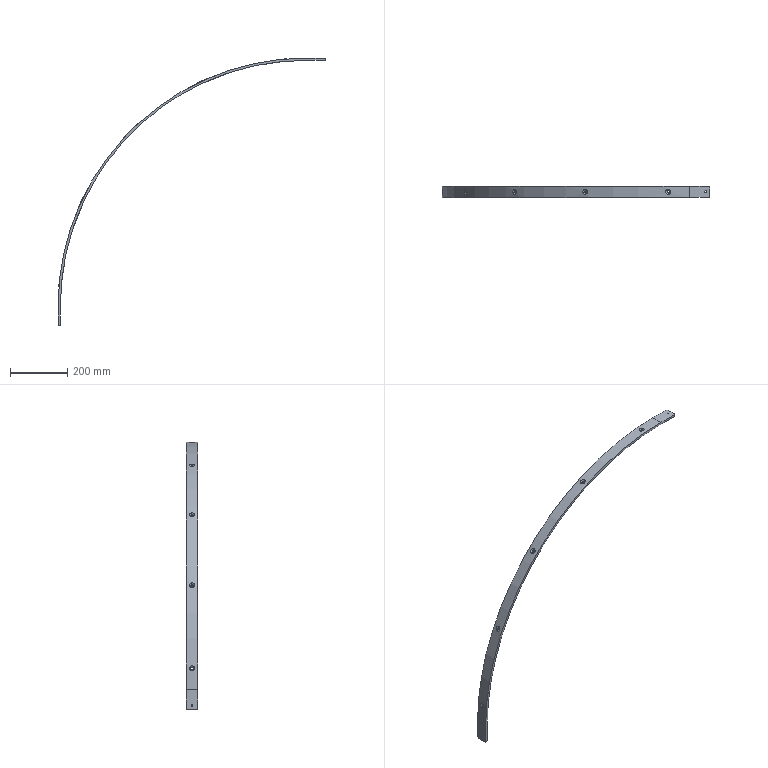Part | STEP file | for inner bend roller | 1 solid | 26 faces | box 938 x 40 x 938 mm | volume 473961 mm3 | plane 12 | spline 6 | cylinder 5 | cone 3 | commonest cylinder face diameters 9 x3 1720 x1 1736 x1